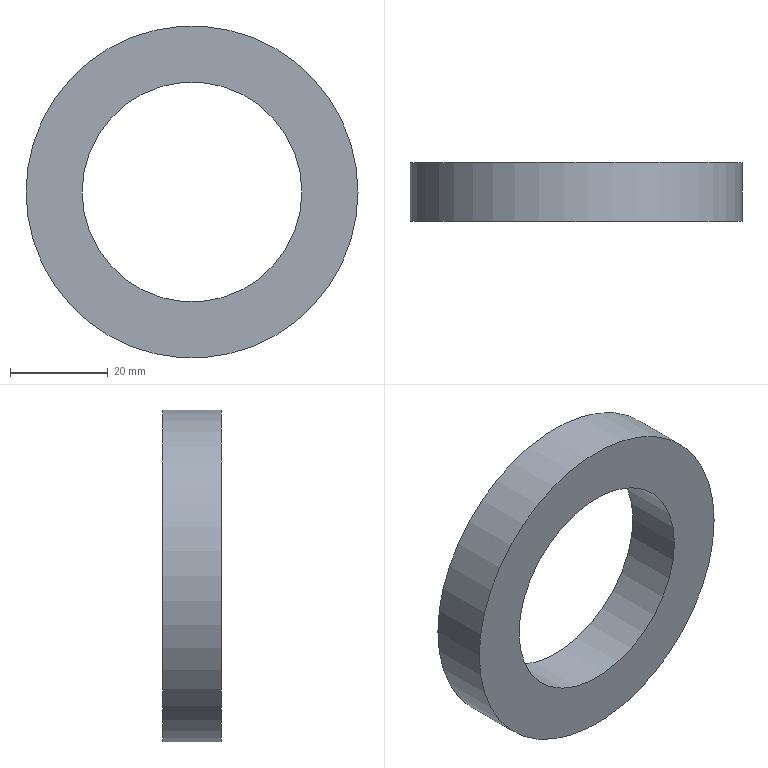Part | NX | features DATUM_CSYS 2, EXTRUDE 1, SKETCH 1 | 1 solid | 4 faces | box 68 x 12 x 68 mm | volume 24495 mm3 | cylinder 2 | plane 2 | commonest cylinder face diameters 45 x1 68 x1
STEP:
#1=CARTESIAN_POINT('',(34.,-12.,0.));
#2=VERTEX_POINT('',#1);
#3=CARTESIAN_POINT('',(0.,-12.,0.));
#4=DIRECTION('',(0.,-1.,0.));
#5=DIRECTION('',(1.,0.,0.));
#6=AXIS2_PLACEMENT_3D('',#3,#4,#5);
#7=CIRCLE('',#6,34.);
#8=EDGE_CURVE('',#2,#2,#7,.T.);
#9=ORIENTED_EDGE('',*,*,#8,.F.);
#10=EDGE_LOOP('',(#9));
#11=FACE_BOUND('',#10,.T.);
#12=CARTESIAN_POINT('',(34.,0.,0.));
#13=VERTEX_POINT('',#12);
#14=CARTESIAN_POINT('',(0.,0.,0.));
#15=DIRECTION('',(0.,-1.,0.));
#16=DIRECTION('',(1.,0.,0.));
#17=AXIS2_PLACEMENT_3D('',#14,#15,#16);
#18=CIRCLE('',#17,34.);
#19=EDGE_CURVE('',#13,#13,#18,.T.);
#20=ORIENTED_EDGE('',*,*,#19,.T.);
#21=EDGE_LOOP('',(#20));
#22=FACE_BOUND('',#21,.T.);
#23=CARTESIAN_POINT('',(0.,-12.,0.));
#24=DIRECTION('',(0.,1.,0.));
#25=DIRECTION('',(0.,0.,1.));
#26=AXIS2_PLACEMENT_3D('',#23,#24,#25);
#27=CYLINDRICAL_SURFACE('',#26,34.);
#28=ADVANCED_FACE('',(#11,#22),#27,.T.);
#29=CARTESIAN_POINT('',(22.5,-12.,0.));
#30=VERTEX_POINT('',#29);
#31=CARTESIAN_POINT('',(0.,-12.,0.));
#32=DIRECTION('',(0.,-1.,0.));
#33=DIRECTION('',(1.,0.,0.));
#34=AXIS2_PLACEMENT_3D('',#31,#32,#33);
#35=CIRCLE('',#34,22.5);
#36=EDGE_CURVE('',#30,#30,#35,.T.);
#37=ORIENTED_EDGE('',*,*,#36,.T.);
#38=EDGE_LOOP('',(#37));
#39=FACE_BOUND('',#38,.T.);
#40=CARTESIAN_POINT('',(22.5,0.,0.));
#41=VERTEX_POINT('',#40);
#42=CARTESIAN_POINT('',(0.,0.,0.));
#43=DIRECTION('',(0.,-1.,0.));
#44=DIRECTION('',(1.,0.,0.));
#45=AXIS2_PLACEMENT_3D('',#42,#43,#44);
#46=CIRCLE('',#45,22.5);
#47=EDGE_CURVE('',#41,#41,#46,.T.);
#48=ORIENTED_EDGE('',*,*,#47,.F.);
#49=EDGE_LOOP('',(#48));
#50=FACE_BOUND('',#49,.T.);
#51=CARTESIAN_POINT('',(0.,-12.,0.));
#52=DIRECTION('',(0.,1.,0.));
#53=DIRECTION('',(0.,0.,1.));
#54=AXIS2_PLACEMENT_3D('',#51,#52,#53);
#55=CYLINDRICAL_SURFACE('',#54,22.5);
#56=ADVANCED_FACE('',(#39,#50),#55,.F.);
#57=ORIENTED_EDGE('',*,*,#8,.T.);
#58=EDGE_LOOP('',(#57));
#59=FACE_BOUND('',#58,.T.);
#60=ORIENTED_EDGE('',*,*,#36,.F.);
#61=EDGE_LOOP('',(#60));
#62=FACE_BOUND('',#61,.T.);
#63=CARTESIAN_POINT('',(0.,-12.,0.));
#64=DIRECTION('',(0.,-1.,0.));
#65=DIRECTION('',(0.,0.,-1.));
#66=AXIS2_PLACEMENT_3D('',#63,#64,#65);
#67=PLANE('',#66);
#68=ADVANCED_FACE('',(#59,#62),#67,.T.);
#69=ORIENTED_EDGE('',*,*,#19,.F.);
#70=EDGE_LOOP('',(#69));
#71=FACE_BOUND('',#70,.T.);
#72=ORIENTED_EDGE('',*,*,#47,.T.);
#73=EDGE_LOOP('',(#72));
#74=FACE_BOUND('',#73,.T.);
#75=CARTESIAN_POINT('',(0.,0.,0.));
#76=DIRECTION('',(0.,-1.,0.));
#77=DIRECTION('',(0.,0.,-1.));
#78=AXIS2_PLACEMENT_3D('',#75,#76,#77);
#79=PLANE('',#78);
#80=ADVANCED_FACE('',(#71,#74),#79,.F.);
#81=CLOSED_SHELL('',(#28,#56,#68,#80));
#82=MANIFOLD_SOLID_BREP('',#81);
#83=(LENGTH_UNIT()NAMED_UNIT(*)SI_UNIT(.MILLI.,.METRE.));
#84=UNCERTAINTY_MEASURE_WITH_UNIT(LENGTH_MEASURE(0.00001),#83,'','');
#85=(NAMED_UNIT(*)PLANE_ANGLE_UNIT()SI_UNIT($,.RADIAN.));
#86=(NAMED_UNIT(*)SI_UNIT($,.STERADIAN.)SOLID_ANGLE_UNIT());
#87=(GEOMETRIC_REPRESENTATION_CONTEXT(3)GLOBAL_UNCERTAINTY_ASSIGNED_CONTEXT((#84))GLOBAL_UNIT_ASSIGNED_CONTEXT((#83,#85,#86))REPRESENTATION_CONTEXT('',''));
#88=ADVANCED_BREP_SHAPE_REPRESENTATION('',(#82),#87);